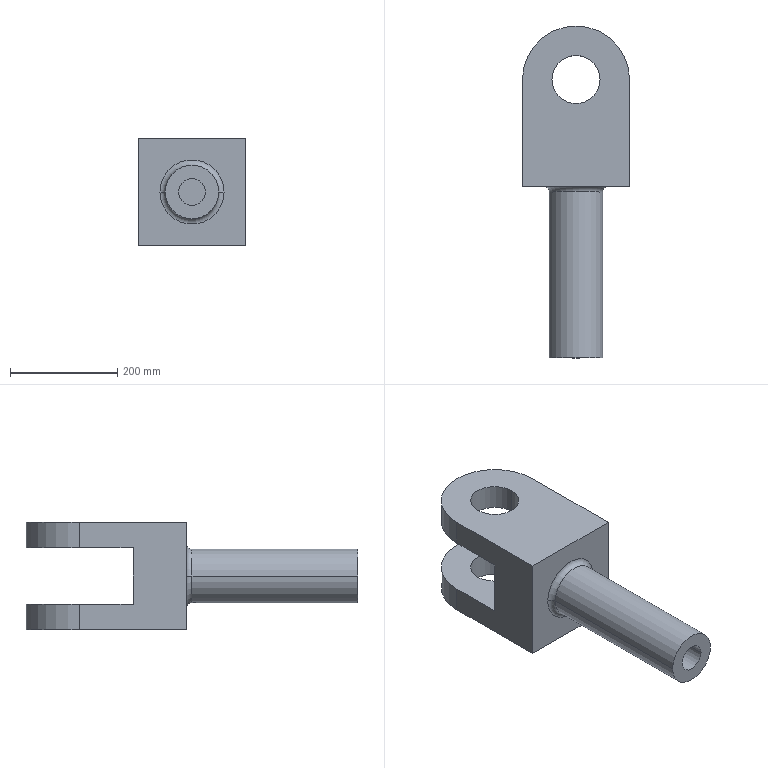Part | SolidWorks | features ICE 3, Extrusion 1, Fillet 1 | 1 solid | 22 faces | box 200 x 620 x 200 mm | volume 9111860 mm3 | cylinder 10 | plane 10 | torus 2 | commonest cylinder face diameters 90 x4 50 x2 100 x2 200 x2
STEP:
#1=CARTESIAN_POINT('',(100.402,-159.598,100.));
#2=VERTEX_POINT('',#1);
#3=CARTESIAN_POINT('',(-19.598,-159.598,100.));
#4=VERTEX_POINT('',#3);
#5=CARTESIAN_POINT('',(40.402,-159.598,100.));
#6=DIRECTION('',(0.,1.,0.));
#7=DIRECTION('',(-1.,0.,0.));
#8=AXIS2_PLACEMENT_3D('',#5,#6,#7);
#9=CIRCLE('',#8,60.);
#10=EDGE_CURVE('',#2,#4,#9,.T.);
#11=ORIENTED_EDGE('',*,*,#10,.F.);
#12=CARTESIAN_POINT('',(90.402,-169.598,100.));
#13=VERTEX_POINT('',#12);
#14=CARTESIAN_POINT('',(100.402,-169.598,100.));
#15=DIRECTION('',(0.,0.,1.));
#16=DIRECTION('',(1.,0.,0.));
#17=AXIS2_PLACEMENT_3D('',#14,#15,#16);
#18=CIRCLE('',#17,10.);
#19=EDGE_CURVE('',#2,#13,#18,.T.);
#20=ORIENTED_EDGE('',*,*,#19,.T.);
#21=CARTESIAN_POINT('',(-9.598,-169.598,100.));
#22=VERTEX_POINT('',#21);
#23=CARTESIAN_POINT('',(40.402,-169.598,100.));
#24=DIRECTION('',(0.,-1.,0.));
#25=DIRECTION('',(-1.,0.,0.));
#26=AXIS2_PLACEMENT_3D('',#23,#24,#25);
#27=CIRCLE('',#26,50.);
#28=EDGE_CURVE('',#22,#13,#27,.T.);
#29=ORIENTED_EDGE('',*,*,#28,.F.);
#30=CARTESIAN_POINT('',(-19.598,-169.598,100.));
#31=DIRECTION('',(0.,0.,-1.));
#32=DIRECTION('',(-1.,0.,0.));
#33=AXIS2_PLACEMENT_3D('',#30,#31,#32);
#34=CIRCLE('',#33,10.);
#35=EDGE_CURVE('',#4,#22,#34,.T.);
#36=ORIENTED_EDGE('',*,*,#35,.F.);
#37=EDGE_LOOP('',(#11,#20,#29,#36));
#38=FACE_OUTER_BOUND('',#37,.T.);
#39=CARTESIAN_POINT('',(40.402,-169.598,100.));
#40=DIRECTION('',(0.,1.,0.));
#41=DIRECTION('',(-1.,0.,0.));
#42=AXIS2_PLACEMENT_3D('',#39,#40,#41);
#43=TOROIDAL_SURFACE('',#42,60.,10.);
#44=ADVANCED_FACE('',(#38),#43,.F.);
#45=CARTESIAN_POINT('',(15.402,-379.598,100.));
#46=VERTEX_POINT('',#45);
#47=CARTESIAN_POINT('',(65.402,-379.598,100.));
#48=VERTEX_POINT('',#47);
#49=CARTESIAN_POINT('',(40.402,-379.598,100.));
#50=DIRECTION('',(0.,-1.,0.));
#51=DIRECTION('',(1.,0.,0.));
#52=AXIS2_PLACEMENT_3D('',#49,#50,#51);
#53=CIRCLE('',#52,25.);
#54=EDGE_CURVE('',#46,#48,#53,.T.);
#55=ORIENTED_EDGE('',*,*,#54,.F.);
#56=CARTESIAN_POINT('',(15.402,-479.598,100.));
#57=VERTEX_POINT('',#56);
#58=CARTESIAN_POINT('',(15.402,-379.598,100.));
#59=DIRECTION('',(0.,-1.,0.));
#60=VECTOR('',#59,1000.);
#61=LINE('',#58,#60);
#62=EDGE_CURVE('',#46,#57,#61,.T.);
#63=ORIENTED_EDGE('',*,*,#62,.T.);
#64=CARTESIAN_POINT('',(65.402,-479.598,100.));
#65=VERTEX_POINT('',#64);
#66=CARTESIAN_POINT('',(40.402,-479.598,100.));
#67=DIRECTION('',(0.,-1.,0.));
#68=DIRECTION('',(1.,0.,0.));
#69=AXIS2_PLACEMENT_3D('',#66,#67,#68);
#70=CIRCLE('',#69,25.);
#71=EDGE_CURVE('',#57,#65,#70,.T.);
#72=ORIENTED_EDGE('',*,*,#71,.T.);
#73=CARTESIAN_POINT('',(65.402,-379.598,100.));
#74=DIRECTION('',(0.,-1.,0.));
#75=VECTOR('',#74,1000.);
#76=LINE('',#73,#75);
#77=EDGE_CURVE('',#48,#65,#76,.T.);
#78=ORIENTED_EDGE('',*,*,#77,.F.);
#79=EDGE_LOOP('',(#55,#63,#72,#78));
#80=FACE_OUTER_BOUND('',#79,.T.);
#81=CARTESIAN_POINT('',(40.402,-379.598,100.));
#82=DIRECTION('',(0.,-1.,0.));
#83=DIRECTION('',(1.,0.,0.));
#84=AXIS2_PLACEMENT_3D('',#81,#82,#83);
#85=CYLINDRICAL_SURFACE('',#84,25.);
#86=ADVANCED_FACE('',(#80),#85,.F.);
#87=CARTESIAN_POINT('',(90.402,-479.598,100.));
#88=VERTEX_POINT('',#87);
#89=CARTESIAN_POINT('',(-9.598,-479.598,100.));
#90=VERTEX_POINT('',#89);
#91=CARTESIAN_POINT('',(40.402,-479.598,100.));
#92=DIRECTION('',(0.,-1.,0.));
#93=DIRECTION('',(1.,0.,0.));
#94=AXIS2_PLACEMENT_3D('',#91,#92,#93);
#95=CIRCLE('',#94,50.);
#96=EDGE_CURVE('',#88,#90,#95,.T.);
#97=ORIENTED_EDGE('',*,*,#96,.F.);
#98=CARTESIAN_POINT('',(90.402,-479.598,100.));
#99=DIRECTION('',(0.,1.,0.));
#100=VECTOR('',#99,1000.);
#101=LINE('',#98,#100);
#102=EDGE_CURVE('',#88,#13,#101,.T.);
#103=ORIENTED_EDGE('',*,*,#102,.T.);
#104=CARTESIAN_POINT('',(40.402,-169.598,100.));
#105=DIRECTION('',(0.,-1.,0.));
#106=DIRECTION('',(-1.,0.,0.));
#107=AXIS2_PLACEMENT_3D('',#104,#105,#106);
#108=CIRCLE('',#107,50.);
#109=EDGE_CURVE('',#13,#22,#108,.T.);
#110=ORIENTED_EDGE('',*,*,#109,.T.);
#111=CARTESIAN_POINT('',(-9.598,-479.598,100.));
#112=DIRECTION('',(0.,1.,0.));
#113=VECTOR('',#112,1000.);
#114=LINE('',#111,#113);
#115=EDGE_CURVE('',#90,#22,#114,.T.);
#116=ORIENTED_EDGE('',*,*,#115,.F.);
#117=EDGE_LOOP('',(#97,#103,#110,#116));
#118=FACE_OUTER_BOUND('',#117,.T.);
#119=CARTESIAN_POINT('',(40.402,-479.598,100.));
#120=DIRECTION('',(0.,1.,0.));
#121=DIRECTION('',(-1.,0.,0.));
#122=AXIS2_PLACEMENT_3D('',#119,#120,#121);
#123=CYLINDRICAL_SURFACE('',#122,50.);
#124=ADVANCED_FACE('',(#118),#123,.T.);
#125=CARTESIAN_POINT('',(-4.598,40.402,200.));
#126=VERTEX_POINT('',#125);
#127=CARTESIAN_POINT('',(85.402,40.402,200.));
#128=VERTEX_POINT('',#127);
#129=CARTESIAN_POINT('',(40.402,40.402,200.));
#130=DIRECTION('',(0.,0.,1.));
#131=DIRECTION('',(1.,0.,0.));
#132=AXIS2_PLACEMENT_3D('',#129,#130,#131);
#133=CIRCLE('',#132,45.);
#134=EDGE_CURVE('',#126,#128,#133,.T.);
#135=ORIENTED_EDGE('',*,*,#134,.T.);
#136=CARTESIAN_POINT('',(85.402,40.402,152.5));
#137=VERTEX_POINT('',#136);
#138=CARTESIAN_POINT('',(85.402,40.402,200.));
#139=DIRECTION('',(0.,0.,-1.));
#140=VECTOR('',#139,1000.);
#141=LINE('',#138,#140);
#142=EDGE_CURVE('',#128,#137,#141,.T.);
#143=ORIENTED_EDGE('',*,*,#142,.T.);
#144=CARTESIAN_POINT('',(-4.598,40.402,152.5));
#145=VERTEX_POINT('',#144);
#146=CARTESIAN_POINT('',(40.402,40.402,152.5));
#147=DIRECTION('',(0.,0.,1.));
#148=DIRECTION('',(0.,-1.,0.));
#149=AXIS2_PLACEMENT_3D('',#146,#147,#148);
#150=CIRCLE('',#149,45.);
#151=EDGE_CURVE('',#145,#137,#150,.T.);
#152=ORIENTED_EDGE('',*,*,#151,.F.);
#153=CARTESIAN_POINT('',(-4.598,40.402,200.));
#154=DIRECTION('',(0.,0.,-1.));
#155=VECTOR('',#154,1000.);
#156=LINE('',#153,#155);
#157=EDGE_CURVE('',#126,#145,#156,.T.);
#158=ORIENTED_EDGE('',*,*,#157,.F.);
#159=EDGE_LOOP('',(#135,#143,#152,#158));
#160=FACE_OUTER_BOUND('',#159,.T.);
#161=CARTESIAN_POINT('',(40.402,40.402,200.));
#162=DIRECTION('',(0.,0.,-1.));
#163=DIRECTION('',(-1.,0.,0.));
#164=AXIS2_PLACEMENT_3D('',#161,#162,#163);
#165=CYLINDRICAL_SURFACE('',#164,45.);
#166=ADVANCED_FACE('',(#160),#165,.F.);
#167=CARTESIAN_POINT('',(85.402,40.402,47.5));
#168=VERTEX_POINT('',#167);
#169=CARTESIAN_POINT('',(-4.598,40.402,47.5));
#170=VERTEX_POINT('',#169);
#171=CARTESIAN_POINT('',(40.402,40.402,47.5));
#172=DIRECTION('',(0.,0.,-1.));
#173=DIRECTION('',(0.,1.,0.));
#174=AXIS2_PLACEMENT_3D('',#171,#172,#173);
#175=CIRCLE('',#174,45.);
#176=EDGE_CURVE('',#168,#170,#175,.T.);
#177=ORIENTED_EDGE('',*,*,#176,.F.);
#178=CARTESIAN_POINT('',(85.402,40.402,0.));
#179=VERTEX_POINT('',#178);
#180=CARTESIAN_POINT('',(85.402,40.402,200.));
#181=DIRECTION('',(0.,0.,-1.));
#182=VECTOR('',#181,1000.);
#183=LINE('',#180,#182);
#184=EDGE_CURVE('',#168,#179,#183,.T.);
#185=ORIENTED_EDGE('',*,*,#184,.T.);
#186=CARTESIAN_POINT('',(-4.598,40.402,0.));
#187=VERTEX_POINT('',#186);
#188=CARTESIAN_POINT('',(40.402,40.402,0.));
#189=DIRECTION('',(0.,0.,1.));
#190=DIRECTION('',(1.,0.,0.));
#191=AXIS2_PLACEMENT_3D('',#188,#189,#190);
#192=CIRCLE('',#191,45.);
#193=EDGE_CURVE('',#187,#179,#192,.T.);
#194=ORIENTED_EDGE('',*,*,#193,.F.);
#195=CARTESIAN_POINT('',(-4.598,40.402,200.));
#196=DIRECTION('',(0.,0.,-1.));
#197=VECTOR('',#196,1000.);
#198=LINE('',#195,#197);
#199=EDGE_CURVE('',#170,#187,#198,.T.);
#200=ORIENTED_EDGE('',*,*,#199,.F.);
#201=EDGE_LOOP('',(#177,#185,#194,#200));
#202=FACE_OUTER_BOUND('',#201,.T.);
#203=CARTESIAN_POINT('',(40.402,40.402,200.));
#204=DIRECTION('',(0.,0.,-1.));
#205=DIRECTION('',(-1.,0.,0.));
#206=AXIS2_PLACEMENT_3D('',#203,#204,#205);
#207=CYLINDRICAL_SURFACE('',#206,45.);
#208=ADVANCED_FACE('',(#202),#207,.F.);
#209=CARTESIAN_POINT('',(-59.598,40.402,47.5));
#210=VERTEX_POINT('',#209);
#211=CARTESIAN_POINT('',(-59.598,40.402,0.));
#212=VERTEX_POINT('',#211);
#213=CARTESIAN_POINT('',(-59.598,40.402,200.));
#214=DIRECTION('',(0.,0.,-1.));
#215=VECTOR('',#214,1000.);
#216=LINE('',#213,#215);
#217=EDGE_CURVE('',#210,#212,#216,.T.);
#218=ORIENTED_EDGE('',*,*,#217,.F.);
#219=CARTESIAN_POINT('',(140.402,40.402,47.5));
#220=VERTEX_POINT('',#219);
#221=CARTESIAN_POINT('',(40.402,40.402,47.5));
#222=DIRECTION('',(0.,0.,-1.));
#223=DIRECTION('',(0.,1.,0.));
#224=AXIS2_PLACEMENT_3D('',#221,#222,#223);
#225=CIRCLE('',#224,100.);
#226=EDGE_CURVE('',#210,#220,#225,.T.);
#227=ORIENTED_EDGE('',*,*,#226,.T.);
#228=CARTESIAN_POINT('',(140.402,40.402,0.));
#229=VERTEX_POINT('',#228);
#230=CARTESIAN_POINT('',(140.402,40.402,200.));
#231=DIRECTION('',(0.,0.,-1.));
#232=VECTOR('',#231,1000.);
#233=LINE('',#230,#232);
#234=EDGE_CURVE('',#220,#229,#233,.T.);
#235=ORIENTED_EDGE('',*,*,#234,.T.);
#236=CARTESIAN_POINT('',(40.402,40.402,0.));
#237=DIRECTION('',(0.,0.,1.));
#238=DIRECTION('',(1.,0.,0.));
#239=AXIS2_PLACEMENT_3D('',#236,#237,#238);
#240=CIRCLE('',#239,100.);
#241=EDGE_CURVE('',#229,#212,#240,.T.);
#242=ORIENTED_EDGE('',*,*,#241,.T.);
#243=EDGE_LOOP('',(#218,#227,#235,#242));
#244=FACE_OUTER_BOUND('',#243,.T.);
#245=CARTESIAN_POINT('',(40.402,40.402,200.));
#246=DIRECTION('',(0.,0.,-1.));
#247=DIRECTION('',(-1.,0.,0.));
#248=AXIS2_PLACEMENT_3D('',#245,#246,#247);
#249=CYLINDRICAL_SURFACE('',#248,100.);
#250=ADVANCED_FACE('',(#244),#249,.T.);
#251=ORIENTED_EDGE('',*,*,#184,.F.);
#252=CARTESIAN_POINT('',(40.402,40.402,47.5));
#253=DIRECTION('',(0.,0.,-1.));
#254=DIRECTION('',(0.,1.,0.));
#255=AXIS2_PLACEMENT_3D('',#252,#253,#254);
#256=CIRCLE('',#255,45.);
#257=EDGE_CURVE('',#170,#168,#256,.T.);
#258=ORIENTED_EDGE('',*,*,#257,.F.);
#259=ORIENTED_EDGE('',*,*,#199,.T.);
#260=CARTESIAN_POINT('',(40.402,40.402,0.));
#261=DIRECTION('',(0.,0.,1.));
#262=DIRECTION('',(1.,0.,0.));
#263=AXIS2_PLACEMENT_3D('',#260,#261,#262);
#264=CIRCLE('',#263,45.);
#265=EDGE_CURVE('',#179,#187,#264,.T.);
#266=ORIENTED_EDGE('',*,*,#265,.F.);
#267=EDGE_LOOP('',(#251,#258,#259,#266));
#268=FACE_OUTER_BOUND('',#267,.T.);
#269=CARTESIAN_POINT('',(40.402,40.402,200.));
#270=DIRECTION('',(0.,0.,-1.));
#271=DIRECTION('',(-1.,0.,0.));
#272=AXIS2_PLACEMENT_3D('',#269,#270,#271);
#273=CYLINDRICAL_SURFACE('',#272,45.);
#274=ADVANCED_FACE('',(#268),#273,.F.);
#275=CARTESIAN_POINT('',(140.402,40.402,200.));
#276=VERTEX_POINT('',#275);
#277=CARTESIAN_POINT('',(-59.598,40.402,200.));
#278=VERTEX_POINT('',#277);
#279=CARTESIAN_POINT('',(40.402,40.402,200.));
#280=DIRECTION('',(0.,0.,1.));
#281=DIRECTION('',(1.,0.,0.));
#282=AXIS2_PLACEMENT_3D('',#279,#280,#281);
#283=CIRCLE('',#282,100.);
#284=EDGE_CURVE('',#276,#278,#283,.T.);
#285=ORIENTED_EDGE('',*,*,#284,.T.);
#286=CARTESIAN_POINT('',(-59.598,-159.598,200.));
#287=VERTEX_POINT('',#286);
#288=CARTESIAN_POINT('',(-59.598,-159.598,200.));
#289=DIRECTION('',(0.,-1.,0.));
#290=VECTOR('',#289,1000.);
#291=LINE('',#288,#290);
#292=EDGE_CURVE('',#278,#287,#291,.T.);
#293=ORIENTED_EDGE('',*,*,#292,.T.);
#294=CARTESIAN_POINT('',(140.402,-159.598,200.));
#295=VERTEX_POINT('',#294);
#296=CARTESIAN_POINT('',(140.402,-159.598,200.));
#297=DIRECTION('',(1.,0.,0.));
#298=VECTOR('',#297,1000.);
#299=LINE('',#296,#298);
#300=EDGE_CURVE('',#287,#295,#299,.T.);
#301=ORIENTED_EDGE('',*,*,#300,.T.);
#302=CARTESIAN_POINT('',(140.402,-159.598,200.));
#303=DIRECTION('',(0.,1.,0.));
#304=VECTOR('',#303,1000.);
#305=LINE('',#302,#304);
#306=EDGE_CURVE('',#295,#276,#305,.T.);
#307=ORIENTED_EDGE('',*,*,#306,.T.);
#308=EDGE_LOOP('',(#285,#293,#301,#307));
#309=FACE_OUTER_BOUND('',#308,.T.);
#310=ORIENTED_EDGE('',*,*,#134,.F.);
#311=CARTESIAN_POINT('',(40.402,40.402,200.));
#312=DIRECTION('',(0.,0.,1.));
#313=DIRECTION('',(1.,0.,0.));
#314=AXIS2_PLACEMENT_3D('',#311,#312,#313);
#315=CIRCLE('',#314,45.);
#316=EDGE_CURVE('',#128,#126,#315,.T.);
#317=ORIENTED_EDGE('',*,*,#316,.F.);
#318=EDGE_LOOP('',(#310,#317));
#319=FACE_BOUND('',#318,.T.);
#320=CARTESIAN_POINT('',(40.402,40.402,200.));
#321=DIRECTION('',(0.,0.,1.));
#322=DIRECTION('',(1.,0.,0.));
#323=AXIS2_PLACEMENT_3D('',#320,#321,#322);
#324=PLANE('',#323);
#325=ADVANCED_FACE('',(#309,#319),#324,.T.);
#326=ORIENTED_EDGE('',*,*,#241,.F.);
#327=CARTESIAN_POINT('',(140.402,-159.598,0.));
#328=VERTEX_POINT('',#327);
#329=CARTESIAN_POINT('',(140.402,-159.598,0.));
#330=DIRECTION('',(0.,1.,0.));
#331=VECTOR('',#330,1000.);
#332=LINE('',#329,#331);
#333=EDGE_CURVE('',#328,#229,#332,.T.);
#334=ORIENTED_EDGE('',*,*,#333,.F.);
#335=CARTESIAN_POINT('',(-59.598,-159.598,0.));
#336=VERTEX_POINT('',#335);
#337=CARTESIAN_POINT('',(140.402,-159.598,0.));
#338=DIRECTION('',(1.,0.,0.));
#339=VECTOR('',#338,1000.);
#340=LINE('',#337,#339);
#341=EDGE_CURVE('',#336,#328,#340,.T.);
#342=ORIENTED_EDGE('',*,*,#341,.F.);
#343=CARTESIAN_POINT('',(-59.598,-159.598,0.));
#344=DIRECTION('',(0.,-1.,0.));
#345=VECTOR('',#344,1000.);
#346=LINE('',#343,#345);
#347=EDGE_CURVE('',#212,#336,#346,.T.);
#348=ORIENTED_EDGE('',*,*,#347,.F.);
#349=EDGE_LOOP('',(#326,#334,#342,#348));
#350=FACE_OUTER_BOUND('',#349,.T.);
#351=ORIENTED_EDGE('',*,*,#193,.T.);
#352=ORIENTED_EDGE('',*,*,#265,.T.);
#353=EDGE_LOOP('',(#351,#352));
#354=FACE_BOUND('',#353,.T.);
#355=CARTESIAN_POINT('',(40.402,40.402,0.));
#356=DIRECTION('',(0.,0.,1.));
#357=DIRECTION('',(1.,0.,0.));
#358=AXIS2_PLACEMENT_3D('',#355,#356,#357);
#359=PLANE('',#358);
#360=ADVANCED_FACE('',(#350,#354),#359,.F.);
#361=CARTESIAN_POINT('',(140.402,40.402,152.5));
#362=VERTEX_POINT('',#361);
#363=CARTESIAN_POINT('',(140.402,40.402,200.));
#364=DIRECTION('',(0.,0.,-1.));
#365=VECTOR('',#364,1000.);
#366=LINE('',#363,#365);
#367=EDGE_CURVE('',#276,#362,#366,.T.);
#368=ORIENTED_EDGE('',*,*,#367,.T.);
#369=CARTESIAN_POINT('',(-59.598,40.402,152.5));
#370=VERTEX_POINT('',#369);
#371=CARTESIAN_POINT('',(40.402,40.402,152.5));
#372=DIRECTION('',(0.,0.,1.));
#373=DIRECTION('',(0.,-1.,0.));
#374=AXIS2_PLACEMENT_3D('',#371,#372,#373);
#375=CIRCLE('',#374,100.);
#376=EDGE_CURVE('',#362,#370,#375,.T.);
#377=ORIENTED_EDGE('',*,*,#376,.T.);
#378=CARTESIAN_POINT('',(-59.598,40.402,200.));
#379=DIRECTION('',(0.,0.,-1.));
#380=VECTOR('',#379,1000.);
#381=LINE('',#378,#380);
#382=EDGE_CURVE('',#278,#370,#381,.T.);
#383=ORIENTED_EDGE('',*,*,#382,.F.);
#384=ORIENTED_EDGE('',*,*,#284,.F.);
#385=EDGE_LOOP('',(#368,#377,#383,#384));
#386=FACE_OUTER_BOUND('',#385,.T.);
#387=CARTESIAN_POINT('',(40.402,40.402,200.));
#388=DIRECTION('',(0.,0.,-1.));
#389=DIRECTION('',(-1.,0.,0.));
#390=AXIS2_PLACEMENT_3D('',#387,#388,#389);
#391=CYLINDRICAL_SURFACE('',#390,100.);
#392=ADVANCED_FACE('',(#386),#391,.T.);
#393=CARTESIAN_POINT('',(-59.598,-59.598,152.5));
#394=VERTEX_POINT('',#393);
#395=CARTESIAN_POINT('',(-59.598,-59.598,47.5));
#396=VERTEX_POINT('',#395);
#397=CARTESIAN_POINT('',(-59.598,-59.598,152.5));
#398=DIRECTION('',(0.,0.,-1.));
#399=VECTOR('',#398,1000.);
#400=LINE('',#397,#399);
#401=EDGE_CURVE('',#394,#396,#400,.T.);
#402=ORIENTED_EDGE('',*,*,#401,.T.);
#403=CARTESIAN_POINT('',(-59.598,258.452,47.5));
#404=DIRECTION('',(0.,1.,0.));
#405=VECTOR('',#404,1000.);
#406=LINE('',#403,#405);
#407=EDGE_CURVE('',#396,#210,#406,.T.);
#408=ORIENTED_EDGE('',*,*,#407,.T.);
#409=ORIENTED_EDGE('',*,*,#217,.T.);
#410=ORIENTED_EDGE('',*,*,#347,.T.);
#411=CARTESIAN_POINT('',(-59.598,-159.598,200.));
#412=DIRECTION('',(0.,0.,-1.));
#413=VECTOR('',#412,1000.);
#414=LINE('',#411,#413);
#415=EDGE_CURVE('',#287,#336,#414,.T.);
#416=ORIENTED_EDGE('',*,*,#415,.F.);
#417=ORIENTED_EDGE('',*,*,#292,.F.);
#418=ORIENTED_EDGE('',*,*,#382,.T.);
#419=CARTESIAN_POINT('',(-59.598,258.452,152.5));
#420=DIRECTION('',(0.,-1.,0.));
#421=VECTOR('',#420,1000.);
#422=LINE('',#419,#421);
#423=EDGE_CURVE('',#370,#394,#422,.T.);
#424=ORIENTED_EDGE('',*,*,#423,.T.);
#425=EDGE_LOOP('',(#402,#408,#409,#410,#416,#417,#418,#424));
#426=FACE_OUTER_BOUND('',#425,.T.);
#427=CARTESIAN_POINT('',(-59.598,-159.598,200.));
#428=DIRECTION('',(1.,0.,0.));
#429=DIRECTION('',(0.,1.,0.));
#430=AXIS2_PLACEMENT_3D('',#427,#428,#429);
#431=PLANE('',#430);
#432=ADVANCED_FACE('',(#426),#431,.F.);
#433=CARTESIAN_POINT('',(40.402,-159.598,100.));
#434=DIRECTION('',(0.,1.,0.));
#435=DIRECTION('',(-1.,0.,0.));
#436=AXIS2_PLACEMENT_3D('',#433,#434,#435);
#437=CIRCLE('',#436,60.);
#438=EDGE_CURVE('',#4,#2,#437,.T.);
#439=ORIENTED_EDGE('',*,*,#438,.T.);
#440=ORIENTED_EDGE('',*,*,#10,.T.);
#441=EDGE_LOOP('',(#439,#440));
#442=FACE_BOUND('',#441,.T.);
#443=ORIENTED_EDGE('',*,*,#341,.T.);
#444=CARTESIAN_POINT('',(140.402,-159.598,200.));
#445=DIRECTION('',(0.,0.,-1.));
#446=VECTOR('',#445,1000.);
#447=LINE('',#444,#446);
#448=EDGE_CURVE('',#295,#328,#447,.T.);
#449=ORIENTED_EDGE('',*,*,#448,.F.);
#450=ORIENTED_EDGE('',*,*,#300,.F.);
#451=ORIENTED_EDGE('',*,*,#415,.T.);
#452=EDGE_LOOP('',(#443,#449,#450,#451));
#453=FACE_OUTER_BOUND('',#452,.T.);
#454=CARTESIAN_POINT('',(140.402,-159.598,200.));
#455=DIRECTION('',(0.,1.,0.));
#456=DIRECTION('',(-1.,0.,0.));
#457=AXIS2_PLACEMENT_3D('',#454,#455,#456);
#458=PLANE('',#457);
#459=ADVANCED_FACE('',(#442,#453),#458,.F.);
#460=ORIENTED_EDGE('',*,*,#234,.F.);
#461=CARTESIAN_POINT('',(140.402,-59.598,47.5));
#462=VERTEX_POINT('',#461);
#463=CARTESIAN_POINT('',(140.402,258.452,47.5));
#464=DIRECTION('',(0.,1.,0.));
#465=VECTOR('',#464,1000.);
#466=LINE('',#463,#465);
#467=EDGE_CURVE('',#462,#220,#466,.T.);
#468=ORIENTED_EDGE('',*,*,#467,.F.);
#469=CARTESIAN_POINT('',(140.402,-59.598,152.5));
#470=VERTEX_POINT('',#469);
#471=CARTESIAN_POINT('',(140.402,-59.598,152.5));
#472=DIRECTION('',(0.,0.,-1.));
#473=VECTOR('',#472,1000.);
#474=LINE('',#471,#473);
#475=EDGE_CURVE('',#470,#462,#474,.T.);
#476=ORIENTED_EDGE('',*,*,#475,.F.);
#477=CARTESIAN_POINT('',(140.402,258.452,152.5));
#478=DIRECTION('',(0.,-1.,0.));
#479=VECTOR('',#478,1000.);
#480=LINE('',#477,#479);
#481=EDGE_CURVE('',#362,#470,#480,.T.);
#482=ORIENTED_EDGE('',*,*,#481,.F.);
#483=ORIENTED_EDGE('',*,*,#367,.F.);
#484=ORIENTED_EDGE('',*,*,#306,.F.);
#485=ORIENTED_EDGE('',*,*,#448,.T.);
#486=ORIENTED_EDGE('',*,*,#333,.T.);
#487=EDGE_LOOP('',(#460,#468,#476,#482,#483,#484,#485,#486));
#488=FACE_OUTER_BOUND('',#487,.T.);
#489=CARTESIAN_POINT('',(140.402,-159.598,200.));
#490=DIRECTION('',(-1.,0.,0.));
#491=DIRECTION('',(0.,0.,1.));
#492=AXIS2_PLACEMENT_3D('',#489,#490,#491);
#493=PLANE('',#492);
#494=ADVANCED_FACE('',(#488),#493,.F.);
#495=ORIENTED_EDGE('',*,*,#142,.F.);
#496=ORIENTED_EDGE('',*,*,#316,.T.);
#497=ORIENTED_EDGE('',*,*,#157,.T.);
#498=CARTESIAN_POINT('',(40.402,40.402,152.5));
#499=DIRECTION('',(0.,0.,1.));
#500=DIRECTION('',(0.,-1.,0.));
#501=AXIS2_PLACEMENT_3D('',#498,#499,#500);
#502=CIRCLE('',#501,45.);
#503=EDGE_CURVE('',#137,#145,#502,.T.);
#504=ORIENTED_EDGE('',*,*,#503,.F.);
#505=EDGE_LOOP('',(#495,#496,#497,#504));
#506=FACE_OUTER_BOUND('',#505,.T.);
#507=CARTESIAN_POINT('',(40.402,40.402,200.));
#508=DIRECTION('',(0.,0.,-1.));
#509=DIRECTION('',(-1.,0.,0.));
#510=AXIS2_PLACEMENT_3D('',#507,#508,#509);
#511=CYLINDRICAL_SURFACE('',#510,45.);
#512=ADVANCED_FACE('',(#506),#511,.F.);
#513=ORIENTED_EDGE('',*,*,#257,.T.);
#514=ORIENTED_EDGE('',*,*,#176,.T.);
#515=EDGE_LOOP('',(#513,#514));
#516=FACE_BOUND('',#515,.T.);
#517=ORIENTED_EDGE('',*,*,#407,.F.);
#518=CARTESIAN_POINT('',(-59.598,-59.598,47.5));
#519=DIRECTION('',(1.,0.,0.));
#520=VECTOR('',#519,1000.);
#521=LINE('',#518,#520);
#522=EDGE_CURVE('',#396,#462,#521,.T.);
#523=ORIENTED_EDGE('',*,*,#522,.T.);
#524=ORIENTED_EDGE('',*,*,#467,.T.);
#525=ORIENTED_EDGE('',*,*,#226,.F.);
#526=EDGE_LOOP('',(#517,#523,#524,#525));
#527=FACE_OUTER_BOUND('',#526,.T.);
#528=CARTESIAN_POINT('',(-59.598,258.452,47.5));
#529=DIRECTION('',(0.,0.,-1.));
#530=DIRECTION('',(0.,1.,0.));
#531=AXIS2_PLACEMENT_3D('',#528,#529,#530);
#532=PLANE('',#531);
#533=ADVANCED_FACE('',(#516,#527),#532,.F.);
#534=ORIENTED_EDGE('',*,*,#151,.T.);
#535=ORIENTED_EDGE('',*,*,#503,.T.);
#536=EDGE_LOOP('',(#534,#535));
#537=FACE_BOUND('',#536,.T.);
#538=ORIENTED_EDGE('',*,*,#481,.T.);
#539=CARTESIAN_POINT('',(-59.598,-59.598,152.5));
#540=DIRECTION('',(1.,0.,0.));
#541=VECTOR('',#540,1000.);
#542=LINE('',#539,#541);
#543=EDGE_CURVE('',#394,#470,#542,.T.);
#544=ORIENTED_EDGE('',*,*,#543,.F.);
#545=ORIENTED_EDGE('',*,*,#423,.F.);
#546=ORIENTED_EDGE('',*,*,#376,.F.);
#547=EDGE_LOOP('',(#538,#544,#545,#546));
#548=FACE_OUTER_BOUND('',#547,.T.);
#549=CARTESIAN_POINT('',(-59.598,258.452,152.5));
#550=DIRECTION('',(0.,0.,1.));
#551=DIRECTION('',(0.,-1.,0.));
#552=AXIS2_PLACEMENT_3D('',#549,#550,#551);
#553=PLANE('',#552);
#554=ADVANCED_FACE('',(#537,#548),#553,.F.);
#555=ORIENTED_EDGE('',*,*,#475,.T.);
#556=ORIENTED_EDGE('',*,*,#522,.F.);
#557=ORIENTED_EDGE('',*,*,#401,.F.);
#558=ORIENTED_EDGE('',*,*,#543,.T.);
#559=EDGE_LOOP('',(#555,#556,#557,#558));
#560=FACE_OUTER_BOUND('',#559,.T.);
#561=CARTESIAN_POINT('',(-59.598,-59.598,152.5));
#562=DIRECTION('',(0.,-1.,0.));
#563=DIRECTION('',(0.,0.,-1.));
#564=AXIS2_PLACEMENT_3D('',#561,#562,#563);
#565=PLANE('',#564);
#566=ADVANCED_FACE('',(#560),#565,.F.);
#567=ORIENTED_EDGE('',*,*,#102,.F.);
#568=CARTESIAN_POINT('',(40.402,-479.598,100.));
#569=DIRECTION('',(0.,-1.,0.));
#570=DIRECTION('',(1.,0.,0.));
#571=AXIS2_PLACEMENT_3D('',#568,#569,#570);
#572=CIRCLE('',#571,50.);
#573=EDGE_CURVE('',#90,#88,#572,.T.);
#574=ORIENTED_EDGE('',*,*,#573,.F.);
#575=ORIENTED_EDGE('',*,*,#115,.T.);
#576=ORIENTED_EDGE('',*,*,#28,.T.);
#577=EDGE_LOOP('',(#567,#574,#575,#576));
#578=FACE_OUTER_BOUND('',#577,.T.);
#579=CARTESIAN_POINT('',(40.402,-479.598,100.));
#580=DIRECTION('',(0.,1.,0.));
#581=DIRECTION('',(-1.,0.,0.));
#582=AXIS2_PLACEMENT_3D('',#579,#580,#581);
#583=CYLINDRICAL_SURFACE('',#582,50.);
#584=ADVANCED_FACE('',(#578),#583,.T.);
#585=CARTESIAN_POINT('',(40.402,-479.598,100.));
#586=DIRECTION('',(0.,-1.,0.));
#587=DIRECTION('',(1.,0.,0.));
#588=AXIS2_PLACEMENT_3D('',#585,#586,#587);
#589=CIRCLE('',#588,25.);
#590=EDGE_CURVE('',#65,#57,#589,.T.);
#591=ORIENTED_EDGE('',*,*,#590,.F.);
#592=ORIENTED_EDGE('',*,*,#71,.F.);
#593=EDGE_LOOP('',(#591,#592));
#594=FACE_BOUND('',#593,.T.);
#595=ORIENTED_EDGE('',*,*,#573,.T.);
#596=ORIENTED_EDGE('',*,*,#96,.T.);
#597=EDGE_LOOP('',(#595,#596));
#598=FACE_OUTER_BOUND('',#597,.T.);
#599=CARTESIAN_POINT('',(40.402,-479.598,100.));
#600=DIRECTION('',(0.,-1.,0.));
#601=DIRECTION('',(1.,0.,0.));
#602=AXIS2_PLACEMENT_3D('',#599,#600,#601);
#603=PLANE('',#602);
#604=ADVANCED_FACE('',(#594,#598),#603,.T.);
#605=ORIENTED_EDGE('',*,*,#62,.F.);
#606=CARTESIAN_POINT('',(40.402,-379.598,100.));
#607=DIRECTION('',(0.,-1.,0.));
#608=DIRECTION('',(1.,0.,0.));
#609=AXIS2_PLACEMENT_3D('',#606,#607,#608);
#610=CIRCLE('',#609,25.);
#611=EDGE_CURVE('',#48,#46,#610,.T.);
#612=ORIENTED_EDGE('',*,*,#611,.F.);
#613=ORIENTED_EDGE('',*,*,#77,.T.);
#614=ORIENTED_EDGE('',*,*,#590,.T.);
#615=EDGE_LOOP('',(#605,#612,#613,#614));
#616=FACE_OUTER_BOUND('',#615,.T.);
#617=CARTESIAN_POINT('',(40.402,-379.598,100.));
#618=DIRECTION('',(0.,-1.,0.));
#619=DIRECTION('',(1.,0.,0.));
#620=AXIS2_PLACEMENT_3D('',#617,#618,#619);
#621=CYLINDRICAL_SURFACE('',#620,25.);
#622=ADVANCED_FACE('',(#616),#621,.F.);
#623=ORIENTED_EDGE('',*,*,#611,.T.);
#624=ORIENTED_EDGE('',*,*,#54,.T.);
#625=EDGE_LOOP('',(#623,#624));
#626=FACE_OUTER_BOUND('',#625,.T.);
#627=CARTESIAN_POINT('',(40.402,-379.598,100.));
#628=DIRECTION('',(0.,-1.,0.));
#629=DIRECTION('',(1.,0.,0.));
#630=AXIS2_PLACEMENT_3D('',#627,#628,#629);
#631=PLANE('',#630);
#632=ADVANCED_FACE('',(#626),#631,.T.);
#633=ORIENTED_EDGE('',*,*,#19,.F.);
#634=ORIENTED_EDGE('',*,*,#438,.F.);
#635=ORIENTED_EDGE('',*,*,#35,.T.);
#636=ORIENTED_EDGE('',*,*,#109,.F.);
#637=EDGE_LOOP('',(#633,#634,#635,#636));
#638=FACE_OUTER_BOUND('',#637,.T.);
#639=CARTESIAN_POINT('',(40.402,-169.598,100.));
#640=DIRECTION('',(0.,1.,0.));
#641=DIRECTION('',(-1.,0.,0.));
#642=AXIS2_PLACEMENT_3D('',#639,#640,#641);
#643=TOROIDAL_SURFACE('',#642,60.,10.);
#644=ADVANCED_FACE('',(#638),#643,.F.);
#645=CLOSED_SHELL('',(#44,#86,#124,#166,#208,#250,#274,#325,#360,#392,#432,#459,#494,#512,#533,#554,#566,#584,#604,#622,#632,#644));
#646=MANIFOLD_SOLID_BREP('',#645);
#647=CARTESIAN_POINT('',(0.,0.,0.));
#648=DIRECTION('',(0.,0.,1.));
#649=DIRECTION('',(1.,0.,0.));
#650=AXIS2_PLACEMENT_3D('',#647,#648,#649);
#651=(LENGTH_UNIT()NAMED_UNIT(*)SI_UNIT(.MILLI.,.METRE.));
#652=UNCERTAINTY_MEASURE_WITH_UNIT(LENGTH_MEASURE(0.00001),#651,'','');
#653=(NAMED_UNIT(*)PLANE_ANGLE_UNIT()SI_UNIT($,.RADIAN.));
#654=(NAMED_UNIT(*)SI_UNIT($,.STERADIAN.)SOLID_ANGLE_UNIT());
#655=(GEOMETRIC_REPRESENTATION_CONTEXT(3)GLOBAL_UNCERTAINTY_ASSIGNED_CONTEXT((#652))GLOBAL_UNIT_ASSIGNED_CONTEXT((#651,#653,#654))REPRESENTATION_CONTEXT('',''));
#656=ADVANCED_BREP_SHAPE_REPRESENTATION('',(#646,#650),#655);